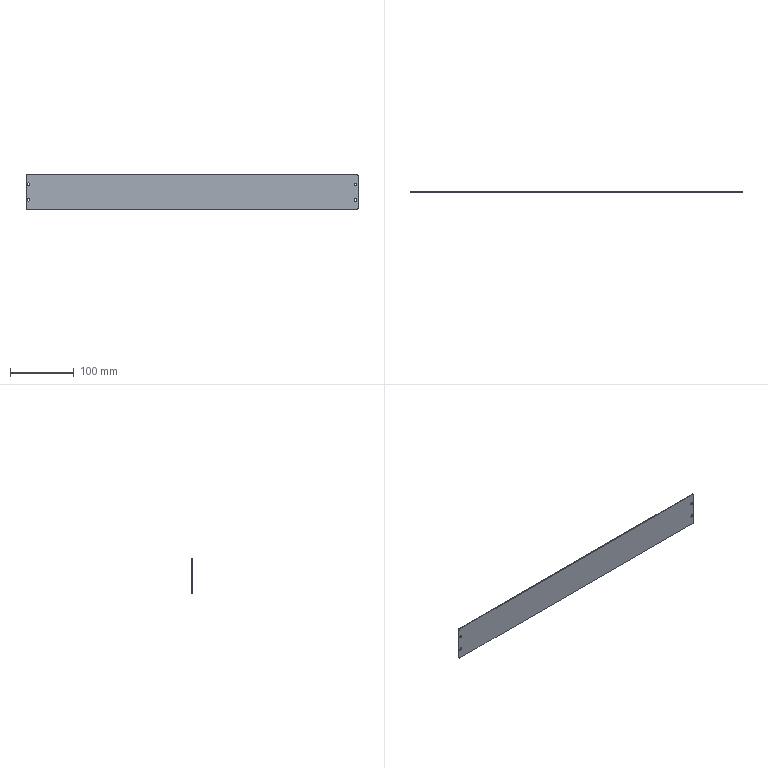Part | STEP file | ASND-0110-TCTF01-30(default) | 1 solid | 22 faces | box 522 x 1.5 x 56 mm | volume 43747 mm3 | cylinder 16 | plane 6 | commonest cylinder face diameters 4 x8 4.5 x8